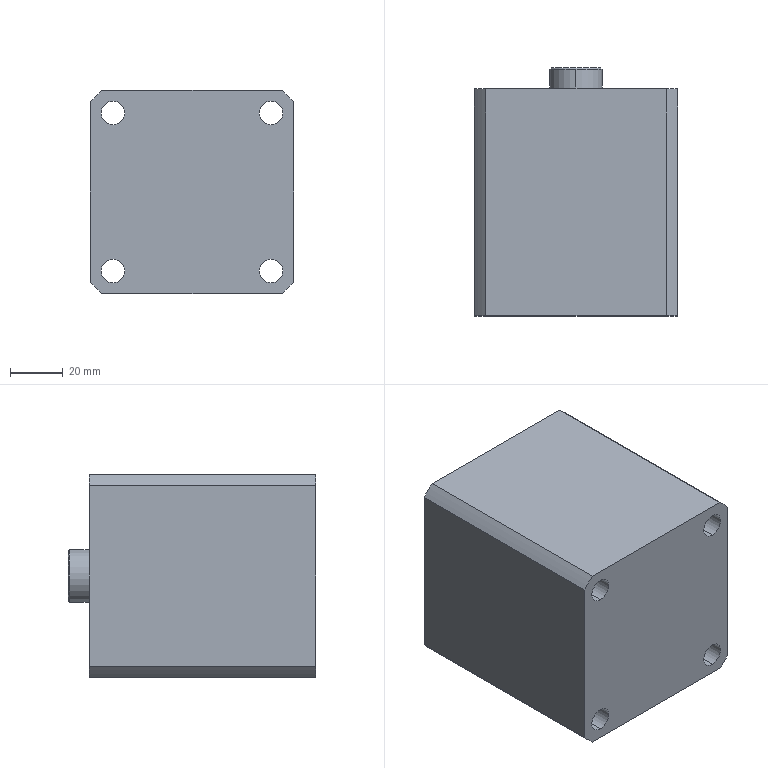Part | STEP file | CDQ2B63-50D-A73 | 1 solid | 29 faces | box 77 x 94 x 77.01 mm | volume 486340 mm3 | cylinder 16 | plane 7 | cone 6 | commonest cylinder face diameters 9 x8 103 x4 8.5 x2 20 x2